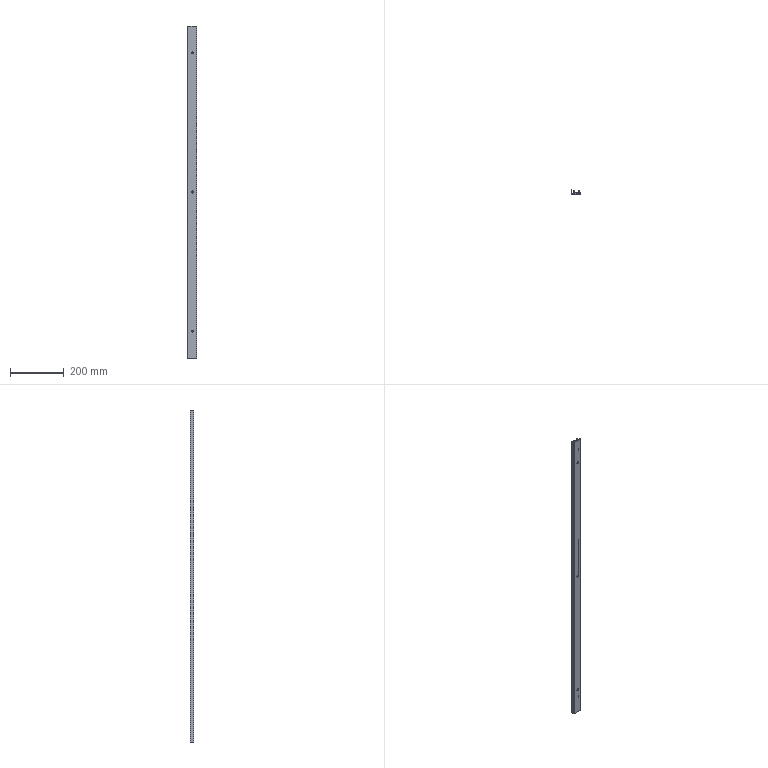Part | SolidWorks | features BaseBody 1, HoleWzd 1, ICE 1, MoveFace 1 | 1 solid | 31 faces | box 33.5 x 13.5 x 1230 mm | volume 229950 mm3 | plane 16 | cylinder 9 | cone 6 | commonest cylinder face diameters 2 x3 13.44 x3 4 x2 1.5 x1
STEP:
#1=CARTESIAN_POINT('',(20.,0.,1033.72));
#2=VERTEX_POINT('',#1);
#3=CARTESIAN_POINT('',(20.,0.,1026.28));
#4=VERTEX_POINT('',#3);
#5=CARTESIAN_POINT('',(20.,0.,1030.));
#6=DIRECTION('',(0.,-1.,0.));
#7=DIRECTION('',(0.,0.,-1.));
#8=AXIS2_PLACEMENT_3D('',#5,#6,#7);
#9=CIRCLE('',#8,3.72);
#10=EDGE_CURVE('',#2,#4,#9,.T.);
#11=ORIENTED_EDGE('',*,*,#10,.T.);
#12=CARTESIAN_POINT('',(20.,3.,1023.28));
#13=VERTEX_POINT('',#12);
#14=CARTESIAN_POINT('',(20.,3.,1023.28));
#15=DIRECTION('',(0.,0.7071,-0.7071));
#16=VECTOR('',#15,1000.);
#17=LINE('',#14,#16);
#18=EDGE_CURVE('',#4,#13,#17,.T.);
#19=ORIENTED_EDGE('',*,*,#18,.T.);
#20=CARTESIAN_POINT('',(20.,3.,1036.72));
#21=VERTEX_POINT('',#20);
#22=CARTESIAN_POINT('',(20.,3.,1030.));
#23=DIRECTION('',(0.,1.,0.));
#24=DIRECTION('',(0.,0.,1.));
#25=AXIS2_PLACEMENT_3D('',#22,#23,#24);
#26=CIRCLE('',#25,6.72);
#27=EDGE_CURVE('',#13,#21,#26,.T.);
#28=ORIENTED_EDGE('',*,*,#27,.T.);
#29=CARTESIAN_POINT('',(20.,3.,1036.72));
#30=DIRECTION('',(0.,0.7071,0.7071));
#31=VECTOR('',#30,1000.);
#32=LINE('',#29,#31);
#33=EDGE_CURVE('',#2,#21,#32,.T.);
#34=ORIENTED_EDGE('',*,*,#33,.F.);
#35=EDGE_LOOP('',(#11,#19,#28,#34));
#36=FACE_OUTER_BOUND('',#35,.T.);
#37=CARTESIAN_POINT('',(20.,3.,1030.));
#38=DIRECTION('',(0.,1.,0.));
#39=DIRECTION('',(0.,0.,1.));
#40=AXIS2_PLACEMENT_3D('',#37,#38,#39);
#41=CONICAL_SURFACE('',#40,6.72,0.7854);
#42=ADVANCED_FACE('',(#36),#41,.F.);
#43=CARTESIAN_POINT('',(20.,0.,3.72));
#44=VERTEX_POINT('',#43);
#45=CARTESIAN_POINT('',(20.,0.,-3.72));
#46=VERTEX_POINT('',#45);
#47=CARTESIAN_POINT('',(20.,0.,0.));
#48=DIRECTION('',(0.,-1.,0.));
#49=DIRECTION('',(0.,0.,-1.));
#50=AXIS2_PLACEMENT_3D('',#47,#48,#49);
#51=CIRCLE('',#50,3.72);
#52=EDGE_CURVE('',#44,#46,#51,.T.);
#53=ORIENTED_EDGE('',*,*,#52,.T.);
#54=CARTESIAN_POINT('',(20.,3.,-6.72));
#55=VERTEX_POINT('',#54);
#56=CARTESIAN_POINT('',(20.,3.,-6.72));
#57=DIRECTION('',(0.,0.7071,-0.7071));
#58=VECTOR('',#57,1000.);
#59=LINE('',#56,#58);
#60=EDGE_CURVE('',#46,#55,#59,.T.);
#61=ORIENTED_EDGE('',*,*,#60,.T.);
#62=CARTESIAN_POINT('',(20.,3.,6.72));
#63=VERTEX_POINT('',#62);
#64=CARTESIAN_POINT('',(20.,3.,0.));
#65=DIRECTION('',(0.,1.,0.));
#66=DIRECTION('',(0.,0.,1.));
#67=AXIS2_PLACEMENT_3D('',#64,#65,#66);
#68=CIRCLE('',#67,6.72);
#69=EDGE_CURVE('',#55,#63,#68,.T.);
#70=ORIENTED_EDGE('',*,*,#69,.T.);
#71=CARTESIAN_POINT('',(20.,3.,6.72));
#72=DIRECTION('',(0.,0.7071,0.7071));
#73=VECTOR('',#72,1000.);
#74=LINE('',#71,#73);
#75=EDGE_CURVE('',#44,#63,#74,.T.);
#76=ORIENTED_EDGE('',*,*,#75,.F.);
#77=EDGE_LOOP('',(#53,#61,#70,#76));
#78=FACE_OUTER_BOUND('',#77,.T.);
#79=CARTESIAN_POINT('',(20.,3.,0.));
#80=DIRECTION('',(0.,1.,0.));
#81=DIRECTION('',(0.,0.,1.));
#82=AXIS2_PLACEMENT_3D('',#79,#80,#81);
#83=CONICAL_SURFACE('',#82,6.72,0.7854);
#84=ADVANCED_FACE('',(#78),#83,.F.);
#85=CARTESIAN_POINT('',(20.,0.,518.72));
#86=VERTEX_POINT('',#85);
#87=CARTESIAN_POINT('',(20.,0.,511.28));
#88=VERTEX_POINT('',#87);
#89=CARTESIAN_POINT('',(20.,0.,515.));
#90=DIRECTION('',(0.,-1.,0.));
#91=DIRECTION('',(0.,0.,-1.));
#92=AXIS2_PLACEMENT_3D('',#89,#90,#91);
#93=CIRCLE('',#92,3.72);
#94=EDGE_CURVE('',#86,#88,#93,.T.);
#95=ORIENTED_EDGE('',*,*,#94,.T.);
#96=CARTESIAN_POINT('',(20.,3.,508.28));
#97=VERTEX_POINT('',#96);
#98=CARTESIAN_POINT('',(20.,3.,508.28));
#99=DIRECTION('',(0.,0.7071,-0.7071));
#100=VECTOR('',#99,1000.);
#101=LINE('',#98,#100);
#102=EDGE_CURVE('',#88,#97,#101,.T.);
#103=ORIENTED_EDGE('',*,*,#102,.T.);
#104=CARTESIAN_POINT('',(20.,3.,521.72));
#105=VERTEX_POINT('',#104);
#106=CARTESIAN_POINT('',(20.,3.,515.));
#107=DIRECTION('',(0.,1.,0.));
#108=DIRECTION('',(0.,0.,1.));
#109=AXIS2_PLACEMENT_3D('',#106,#107,#108);
#110=CIRCLE('',#109,6.72);
#111=EDGE_CURVE('',#97,#105,#110,.T.);
#112=ORIENTED_EDGE('',*,*,#111,.T.);
#113=CARTESIAN_POINT('',(20.,3.,521.72));
#114=DIRECTION('',(0.,0.7071,0.7071));
#115=VECTOR('',#114,1000.);
#116=LINE('',#113,#115);
#117=EDGE_CURVE('',#86,#105,#116,.T.);
#118=ORIENTED_EDGE('',*,*,#117,.F.);
#119=EDGE_LOOP('',(#95,#103,#112,#118));
#120=FACE_OUTER_BOUND('',#119,.T.);
#121=CARTESIAN_POINT('',(20.,3.,515.));
#122=DIRECTION('',(0.,1.,0.));
#123=DIRECTION('',(0.,0.,1.));
#124=AXIS2_PLACEMENT_3D('',#121,#122,#123);
#125=CONICAL_SURFACE('',#124,6.72,0.7854);
#126=ADVANCED_FACE('',(#120),#125,.F.);
#127=CARTESIAN_POINT('',(24.5,10.5,-4.991));
#128=VERTEX_POINT('',#127);
#129=CARTESIAN_POINT('',(24.5,10.5,-100.));
#130=VERTEX_POINT('',#129);
#131=CARTESIAN_POINT('',(24.5,10.5,-100.));
#132=DIRECTION('',(0.,0.,-1.));
#133=VECTOR('',#132,1000.);
#134=LINE('',#131,#133);
#135=EDGE_CURVE('',#128,#130,#134,.T.);
#136=ORIENTED_EDGE('',*,*,#135,.F.);
#137=CARTESIAN_POINT('',(24.5,10.5,4.991));
#138=VERTEX_POINT('',#137);
#139=CARTESIAN_POINT('',(24.5,10.5,-4.991));
#140=CARTESIAN_POINT('',(24.5,10.638,-4.991));
#141=CARTESIAN_POINT('',(24.515,10.777,-4.978));
#142=CARTESIAN_POINT('',(24.57,11.043,-4.927));
#143=CARTESIAN_POINT('',(24.611,11.171,-4.889));
#144=CARTESIAN_POINT('',(24.765,11.529,-4.74));
#145=CARTESIAN_POINT('',(24.907,11.728,-4.597));
#146=CARTESIAN_POINT('',(25.205,12.04,-4.256));
#147=CARTESIAN_POINT('',(25.365,12.156,-4.055));
#148=CARTESIAN_POINT('',(25.663,12.325,-3.627));
#149=CARTESIAN_POINT('',(25.806,12.38,-3.395));
#150=CARTESIAN_POINT('',(26.19,12.494,-2.672));
#151=CARTESIAN_POINT('',(26.387,12.501,-2.161));
#152=CARTESIAN_POINT('',(26.654,12.499,-1.091));
#153=CARTESIAN_POINT('',(26.72,12.488,-0.5481));
#154=CARTESIAN_POINT('',(26.72,12.488,0.2773));
#155=CARTESIAN_POINT('',(26.703,12.49,0.5529));
#156=CARTESIAN_POINT('',(26.636,12.496,1.095));
#157=CARTESIAN_POINT('',(26.586,12.499,1.362));
#158=CARTESIAN_POINT('',(26.388,12.501,2.155));
#159=CARTESIAN_POINT('',(26.188,12.493,2.677));
#160=CARTESIAN_POINT('',(25.805,12.38,3.396));
#161=CARTESIAN_POINT('',(25.662,12.324,3.629));
#162=CARTESIAN_POINT('',(25.438,12.197,3.95));
#163=CARTESIAN_POINT('',(25.362,12.147,4.053));
#164=CARTESIAN_POINT('',(25.208,12.03,4.249));
#165=CARTESIAN_POINT('',(25.13,11.961,4.342));
#166=CARTESIAN_POINT('',(24.98,11.805,4.513));
#167=CARTESIAN_POINT('',(24.908,11.717,4.591));
#168=CARTESIAN_POINT('',(24.774,11.518,4.73));
#169=CARTESIAN_POINT('',(24.714,11.408,4.79));
#170=CARTESIAN_POINT('',(24.612,11.172,4.888));
#171=CARTESIAN_POINT('',(24.57,11.043,4.927));
#172=CARTESIAN_POINT('',(24.515,10.778,4.978));
#173=CARTESIAN_POINT('',(24.5,10.64,4.991));
#174=CARTESIAN_POINT('',(24.5,10.5,4.991));
#175=B_SPLINE_CURVE_WITH_KNOTS('',3,(#139,#140,#141,#142,#143,#144,#145,#146,#147,#148,#149,#150,#151,#152,#153,#154,#155,#156,#157,#158,#159,#160,#161,#162,#163,#164,#165,#166,#167,#168,#169,#170,#171,#172,#173,#174),.UNSPECIFIED.,.F.,.F.,(4,2,2,2,2,2,2,2,2,2,2,2,2,2,2,2,2,4),(0.01321,0.01362,0.01403,0.01486,0.01569,0.01651,0.01816,0.01981,0.02064,0.02146,0.02311,0.02394,0.02435,0.02477,0.02518,0.02559,0.026,0.02642),.UNSPECIFIED.);
#176=EDGE_CURVE('',#128,#138,#175,.T.);
#177=ORIENTED_EDGE('',*,*,#176,.T.);
#178=CARTESIAN_POINT('',(24.5,10.5,510.009));
#179=VERTEX_POINT('',#178);
#180=CARTESIAN_POINT('',(24.5,10.5,-100.));
#181=DIRECTION('',(0.,0.,-1.));
#182=VECTOR('',#181,1000.);
#183=LINE('',#180,#182);
#184=EDGE_CURVE('',#179,#138,#183,.T.);
#185=ORIENTED_EDGE('',*,*,#184,.F.);
#186=CARTESIAN_POINT('',(24.5,10.5,519.991));
#187=VERTEX_POINT('',#186);
#188=CARTESIAN_POINT('',(24.5,10.5,510.009));
#189=CARTESIAN_POINT('',(24.5,10.638,510.009));
#190=CARTESIAN_POINT('',(24.515,10.777,510.022));
#191=CARTESIAN_POINT('',(24.57,11.043,510.073));
#192=CARTESIAN_POINT('',(24.611,11.171,510.111));
#193=CARTESIAN_POINT('',(24.765,11.529,510.26));
#194=CARTESIAN_POINT('',(24.907,11.728,510.403));
#195=CARTESIAN_POINT('',(25.205,12.04,510.744));
#196=CARTESIAN_POINT('',(25.365,12.156,510.945));
#197=CARTESIAN_POINT('',(25.663,12.325,511.373));
#198=CARTESIAN_POINT('',(25.806,12.38,511.605));
#199=CARTESIAN_POINT('',(26.19,12.494,512.328));
#200=CARTESIAN_POINT('',(26.387,12.501,512.839));
#201=CARTESIAN_POINT('',(26.654,12.499,513.909));
#202=CARTESIAN_POINT('',(26.72,12.488,514.452));
#203=CARTESIAN_POINT('',(26.72,12.488,515.277));
#204=CARTESIAN_POINT('',(26.703,12.49,515.553));
#205=CARTESIAN_POINT('',(26.636,12.496,516.095));
#206=CARTESIAN_POINT('',(26.586,12.499,516.362));
#207=CARTESIAN_POINT('',(26.388,12.501,517.155));
#208=CARTESIAN_POINT('',(26.188,12.493,517.677));
#209=CARTESIAN_POINT('',(25.805,12.38,518.396));
#210=CARTESIAN_POINT('',(25.662,12.324,518.629));
#211=CARTESIAN_POINT('',(25.438,12.197,518.95));
#212=CARTESIAN_POINT('',(25.362,12.147,519.053));
#213=CARTESIAN_POINT('',(25.208,12.03,519.249));
#214=CARTESIAN_POINT('',(25.13,11.961,519.342));
#215=CARTESIAN_POINT('',(24.98,11.805,519.513));
#216=CARTESIAN_POINT('',(24.908,11.717,519.591));
#217=CARTESIAN_POINT('',(24.774,11.518,519.73));
#218=CARTESIAN_POINT('',(24.714,11.408,519.79));
#219=CARTESIAN_POINT('',(24.612,11.172,519.888));
#220=CARTESIAN_POINT('',(24.57,11.043,519.927));
#221=CARTESIAN_POINT('',(24.515,10.778,519.978));
#222=CARTESIAN_POINT('',(24.5,10.64,519.991));
#223=CARTESIAN_POINT('',(24.5,10.5,519.991));
#224=B_SPLINE_CURVE_WITH_KNOTS('',3,(#188,#189,#190,#191,#192,#193,#194,#195,#196,#197,#198,#199,#200,#201,#202,#203,#204,#205,#206,#207,#208,#209,#210,#211,#212,#213,#214,#215,#216,#217,#218,#219,#220,#221,#222,#223),.UNSPECIFIED.,.F.,.F.,(4,2,2,2,2,2,2,2,2,2,2,2,2,2,2,2,2,4),(0.01321,0.01362,0.01403,0.01486,0.01569,0.01651,0.01816,0.01981,0.02064,0.02146,0.02311,0.02394,0.02435,0.02477,0.02518,0.02559,0.026,0.02642),.UNSPECIFIED.);
#225=EDGE_CURVE('',#179,#187,#224,.T.);
#226=ORIENTED_EDGE('',*,*,#225,.T.);
#227=CARTESIAN_POINT('',(24.5,10.5,1025.009));
#228=VERTEX_POINT('',#227);
#229=CARTESIAN_POINT('',(24.5,10.5,-100.));
#230=DIRECTION('',(0.,0.,-1.));
#231=VECTOR('',#230,1000.);
#232=LINE('',#229,#231);
#233=EDGE_CURVE('',#228,#187,#232,.T.);
#234=ORIENTED_EDGE('',*,*,#233,.F.);
#235=CARTESIAN_POINT('',(24.5,10.5,1034.991));
#236=VERTEX_POINT('',#235);
#237=CARTESIAN_POINT('',(24.5,10.5,1025.009));
#238=CARTESIAN_POINT('',(24.5,10.64,1025.009));
#239=CARTESIAN_POINT('',(24.514,10.776,1025.022));
#240=CARTESIAN_POINT('',(24.57,11.042,1025.073));
#241=CARTESIAN_POINT('',(24.611,11.171,1025.111));
#242=CARTESIAN_POINT('',(24.713,11.408,1025.209));
#243=CARTESIAN_POINT('',(24.775,11.519,1025.27));
#244=CARTESIAN_POINT('',(24.908,11.717,1025.409));
#245=CARTESIAN_POINT('',(24.981,11.806,1025.488));
#246=CARTESIAN_POINT('',(25.207,12.042,1025.746));
#247=CARTESIAN_POINT('',(25.363,12.155,1025.942));
#248=CARTESIAN_POINT('',(25.665,12.326,1026.376));
#249=CARTESIAN_POINT('',(25.806,12.38,1026.605));
#250=CARTESIAN_POINT('',(26.061,12.456,1027.084));
#251=CARTESIAN_POINT('',(26.176,12.476,1027.337));
#252=CARTESIAN_POINT('',(26.372,12.498,1027.849));
#253=CARTESIAN_POINT('',(26.454,12.501,1028.109));
#254=CARTESIAN_POINT('',(26.586,12.499,1028.638));
#255=CARTESIAN_POINT('',(26.636,12.496,1028.907));
#256=CARTESIAN_POINT('',(26.703,12.49,1029.453));
#257=CARTESIAN_POINT('',(26.72,12.488,1029.729));
#258=CARTESIAN_POINT('',(26.72,12.488,1030.275));
#259=CARTESIAN_POINT('',(26.703,12.49,1030.547));
#260=CARTESIAN_POINT('',(26.637,12.496,1031.089));
#261=CARTESIAN_POINT('',(26.587,12.499,1031.36));
#262=CARTESIAN_POINT('',(26.387,12.501,1032.161));
#263=CARTESIAN_POINT('',(26.191,12.494,1032.671));
#264=CARTESIAN_POINT('',(25.805,12.38,1033.396));
#265=CARTESIAN_POINT('',(25.663,12.325,1033.627));
#266=CARTESIAN_POINT('',(25.364,12.155,1034.057));
#267=CARTESIAN_POINT('',(25.205,12.039,1034.256));
#268=CARTESIAN_POINT('',(24.981,11.805,1034.512));
#269=CARTESIAN_POINT('',(24.907,11.716,1034.592));
#270=CARTESIAN_POINT('',(24.774,11.518,1034.73));
#271=CARTESIAN_POINT('',(24.714,11.409,1034.79));
#272=CARTESIAN_POINT('',(24.611,11.17,1034.889));
#273=CARTESIAN_POINT('',(24.571,11.044,1034.926));
#274=CARTESIAN_POINT('',(24.515,10.78,1034.977));
#275=CARTESIAN_POINT('',(24.5,10.64,1034.991));
#276=CARTESIAN_POINT('',(24.5,10.5,1034.991));
#277=B_SPLINE_CURVE_WITH_KNOTS('',3,(#237,#238,#239,#240,#241,#242,#243,#244,#245,#246,#247,#248,#249,#250,#251,#252,#253,#254,#255,#256,#257,#258,#259,#260,#261,#262,#263,#264,#265,#266,#267,#268,#269,#270,#271,#272,#273,#274,#275,#276),.UNSPECIFIED.,.F.,.F.,(4,2,2,2,2,2,2,2,2,2,2,2,2,2,2,2,2,2,2,4),(0.,0.0004127,0.0008255,0.001238,0.001651,0.002476,0.003302,0.004127,0.004953,0.005778,0.006604,0.007429,0.008255,0.009906,0.01073,0.01156,0.01197,0.01238,0.01279,0.01321),.UNSPECIFIED.);
#278=EDGE_CURVE('',#228,#236,#277,.T.);
#279=ORIENTED_EDGE('',*,*,#278,.T.);
#280=CARTESIAN_POINT('',(24.5,10.5,1130.));
#281=VERTEX_POINT('',#280);
#282=CARTESIAN_POINT('',(24.5,10.5,-100.));
#283=DIRECTION('',(0.,0.,-1.));
#284=VECTOR('',#283,1000.);
#285=LINE('',#282,#284);
#286=EDGE_CURVE('',#281,#236,#285,.T.);
#287=ORIENTED_EDGE('',*,*,#286,.F.);
#288=CARTESIAN_POINT('',(28.5,10.5,1130.));
#289=VERTEX_POINT('',#288);
#290=CARTESIAN_POINT('',(26.5,10.5,1130.));
#291=DIRECTION('',(0.,0.,1.));
#292=DIRECTION('',(1.,0.,0.));
#293=AXIS2_PLACEMENT_3D('',#290,#291,#292);
#294=CIRCLE('',#293,2.);
#295=EDGE_CURVE('',#289,#281,#294,.T.);
#296=ORIENTED_EDGE('',*,*,#295,.F.);
#297=CARTESIAN_POINT('',(28.5,10.5,-100.));
#298=VERTEX_POINT('',#297);
#299=CARTESIAN_POINT('',(28.5,10.5,-100.));
#300=DIRECTION('',(0.,0.,-1.));
#301=VECTOR('',#300,1000.);
#302=LINE('',#299,#301);
#303=EDGE_CURVE('',#289,#298,#302,.T.);
#304=ORIENTED_EDGE('',*,*,#303,.T.);
#305=CARTESIAN_POINT('',(26.5,10.5,-100.));
#306=DIRECTION('',(0.,0.,1.));
#307=DIRECTION('',(-1.,0.,0.));
#308=AXIS2_PLACEMENT_3D('',#305,#306,#307);
#309=CIRCLE('',#308,2.);
#310=EDGE_CURVE('',#298,#130,#309,.T.);
#311=ORIENTED_EDGE('',*,*,#310,.T.);
#312=EDGE_LOOP('',(#136,#177,#185,#226,#234,#279,#287,#296,#304,#311));
#313=FACE_OUTER_BOUND('',#312,.T.);
#314=CARTESIAN_POINT('',(26.5,10.5,-100.));
#315=DIRECTION('',(0.,0.,-1.));
#316=DIRECTION('',(-1.,0.,0.));
#317=AXIS2_PLACEMENT_3D('',#314,#315,#316);
#318=CYLINDRICAL_SURFACE('',#317,2.);
#319=ADVANCED_FACE('',(#313),#318,.T.);
#320=CARTESIAN_POINT('',(24.5,3.,-4.991));
#321=VERTEX_POINT('',#320);
#322=CARTESIAN_POINT('',(24.5,3.,-100.));
#323=VERTEX_POINT('',#322);
#324=CARTESIAN_POINT('',(24.5,3.,-100.));
#325=DIRECTION('',(0.,0.,-1.));
#326=VECTOR('',#325,1000.);
#327=LINE('',#324,#326);
#328=EDGE_CURVE('',#321,#323,#327,.T.);
#329=ORIENTED_EDGE('',*,*,#328,.F.);
#330=CARTESIAN_POINT('',(24.5,13.5,-4.991));
#331=DIRECTION('',(0.,1.,0.));
#332=VECTOR('',#331,1000.);
#333=LINE('',#330,#332);
#334=EDGE_CURVE('',#321,#128,#333,.T.);
#335=ORIENTED_EDGE('',*,*,#334,.T.);
#336=ORIENTED_EDGE('',*,*,#135,.T.);
#337=CARTESIAN_POINT('',(24.5,1.,-100.));
#338=DIRECTION('',(0.,-1.,0.));
#339=VECTOR('',#338,1000.);
#340=LINE('',#337,#339);
#341=EDGE_CURVE('',#130,#323,#340,.T.);
#342=ORIENTED_EDGE('',*,*,#341,.T.);
#343=EDGE_LOOP('',(#329,#335,#336,#342));
#344=FACE_OUTER_BOUND('',#343,.T.);
#345=CARTESIAN_POINT('',(24.5,10.5,-100.));
#346=DIRECTION('',(-1.,0.,0.));
#347=DIRECTION('',(0.,0.,1.));
#348=AXIS2_PLACEMENT_3D('',#345,#346,#347);
#349=PLANE('',#348);
#350=ADVANCED_FACE('',(#344),#349,.T.);
#351=ORIENTED_EDGE('',*,*,#184,.T.);
#352=CARTESIAN_POINT('',(24.5,3.,4.991));
#353=VERTEX_POINT('',#352);
#354=CARTESIAN_POINT('',(24.5,13.5,4.991));
#355=DIRECTION('',(0.,-1.,0.));
#356=VECTOR('',#355,1000.);
#357=LINE('',#354,#356);
#358=EDGE_CURVE('',#138,#353,#357,.T.);
#359=ORIENTED_EDGE('',*,*,#358,.T.);
#360=CARTESIAN_POINT('',(24.5,3.,510.009));
#361=VERTEX_POINT('',#360);
#362=CARTESIAN_POINT('',(24.5,3.,-100.));
#363=DIRECTION('',(0.,0.,-1.));
#364=VECTOR('',#363,1000.);
#365=LINE('',#362,#364);
#366=EDGE_CURVE('',#361,#353,#365,.T.);
#367=ORIENTED_EDGE('',*,*,#366,.F.);
#368=CARTESIAN_POINT('',(24.5,13.5,510.009));
#369=DIRECTION('',(0.,1.,0.));
#370=VECTOR('',#369,1000.);
#371=LINE('',#368,#370);
#372=EDGE_CURVE('',#361,#179,#371,.T.);
#373=ORIENTED_EDGE('',*,*,#372,.T.);
#374=EDGE_LOOP('',(#351,#359,#367,#373));
#375=FACE_OUTER_BOUND('',#374,.T.);
#376=CARTESIAN_POINT('',(24.5,10.5,-100.));
#377=DIRECTION('',(-1.,0.,0.));
#378=DIRECTION('',(0.,0.,1.));
#379=AXIS2_PLACEMENT_3D('',#376,#377,#378);
#380=PLANE('',#379);
#381=ADVANCED_FACE('',(#375),#380,.T.);
#382=ORIENTED_EDGE('',*,*,#233,.T.);
#383=CARTESIAN_POINT('',(24.5,3.,519.991));
#384=VERTEX_POINT('',#383);
#385=CARTESIAN_POINT('',(24.5,13.5,519.991));
#386=DIRECTION('',(0.,-1.,0.));
#387=VECTOR('',#386,1000.);
#388=LINE('',#385,#387);
#389=EDGE_CURVE('',#187,#384,#388,.T.);
#390=ORIENTED_EDGE('',*,*,#389,.T.);
#391=CARTESIAN_POINT('',(24.5,3.,1025.009));
#392=VERTEX_POINT('',#391);
#393=CARTESIAN_POINT('',(24.5,3.,-100.));
#394=DIRECTION('',(0.,0.,-1.));
#395=VECTOR('',#394,1000.);
#396=LINE('',#393,#395);
#397=EDGE_CURVE('',#392,#384,#396,.T.);
#398=ORIENTED_EDGE('',*,*,#397,.F.);
#399=CARTESIAN_POINT('',(24.5,13.5,1025.009));
#400=DIRECTION('',(0.,1.,0.));
#401=VECTOR('',#400,1000.);
#402=LINE('',#399,#401);
#403=EDGE_CURVE('',#392,#228,#402,.T.);
#404=ORIENTED_EDGE('',*,*,#403,.T.);
#405=EDGE_LOOP('',(#382,#390,#398,#404));
#406=FACE_OUTER_BOUND('',#405,.T.);
#407=CARTESIAN_POINT('',(24.5,10.5,-100.));
#408=DIRECTION('',(-1.,0.,0.));
#409=DIRECTION('',(0.,0.,1.));
#410=AXIS2_PLACEMENT_3D('',#407,#408,#409);
#411=PLANE('',#410);
#412=ADVANCED_FACE('',(#406),#411,.T.);
#413=ORIENTED_EDGE('',*,*,#286,.T.);
#414=CARTESIAN_POINT('',(24.5,3.,1034.991));
#415=VERTEX_POINT('',#414);
#416=CARTESIAN_POINT('',(24.5,13.5,1034.991));
#417=DIRECTION('',(0.,-1.,0.));
#418=VECTOR('',#417,1000.);
#419=LINE('',#416,#418);
#420=EDGE_CURVE('',#236,#415,#419,.T.);
#421=ORIENTED_EDGE('',*,*,#420,.T.);
#422=CARTESIAN_POINT('',(24.5,3.,1130.));
#423=VERTEX_POINT('',#422);
#424=CARTESIAN_POINT('',(24.5,3.,-100.));
#425=DIRECTION('',(0.,0.,-1.));
#426=VECTOR('',#425,1000.);
#427=LINE('',#424,#426);
#428=EDGE_CURVE('',#423,#415,#427,.T.);
#429=ORIENTED_EDGE('',*,*,#428,.F.);
#430=CARTESIAN_POINT('',(24.5,1.,1130.));
#431=DIRECTION('',(0.,-1.,0.));
#432=VECTOR('',#431,1000.);
#433=LINE('',#430,#432);
#434=EDGE_CURVE('',#281,#423,#433,.T.);
#435=ORIENTED_EDGE('',*,*,#434,.F.);
#436=EDGE_LOOP('',(#413,#421,#429,#435));
#437=FACE_OUTER_BOUND('',#436,.T.);
#438=CARTESIAN_POINT('',(24.5,10.5,-100.));
#439=DIRECTION('',(-1.,0.,0.));
#440=DIRECTION('',(0.,0.,1.));
#441=AXIS2_PLACEMENT_3D('',#438,#439,#440);
#442=PLANE('',#441);
#443=ADVANCED_FACE('',(#437),#442,.T.);
#444=ORIENTED_EDGE('',*,*,#10,.F.);
#445=CARTESIAN_POINT('',(20.,0.,1030.));
#446=DIRECTION('',(0.,-1.,0.));
#447=DIRECTION('',(0.,0.,-1.));
#448=AXIS2_PLACEMENT_3D('',#445,#446,#447);
#449=CIRCLE('',#448,3.72);
#450=EDGE_CURVE('',#4,#2,#449,.T.);
#451=ORIENTED_EDGE('',*,*,#450,.F.);
#452=EDGE_LOOP('',(#444,#451));
#453=FACE_BOUND('',#452,.T.);
#454=ORIENTED_EDGE('',*,*,#94,.F.);
#455=CARTESIAN_POINT('',(20.,0.,515.));
#456=DIRECTION('',(0.,-1.,0.));
#457=DIRECTION('',(0.,0.,-1.));
#458=AXIS2_PLACEMENT_3D('',#455,#456,#457);
#459=CIRCLE('',#458,3.72);
#460=EDGE_CURVE('',#88,#86,#459,.T.);
#461=ORIENTED_EDGE('',*,*,#460,.F.);
#462=EDGE_LOOP('',(#454,#461));
#463=FACE_BOUND('',#462,.T.);
#464=CARTESIAN_POINT('',(1.,0.,-100.));
#465=VERTEX_POINT('',#464);
#466=CARTESIAN_POINT('',(32.5,0.,-100.));
#467=VERTEX_POINT('',#466);
#468=CARTESIAN_POINT('',(1.,0.,-100.));
#469=DIRECTION('',(1.,0.,0.));
#470=VECTOR('',#469,1000.);
#471=LINE('',#468,#470);
#472=EDGE_CURVE('',#465,#467,#471,.T.);
#473=ORIENTED_EDGE('',*,*,#472,.T.);
#474=CARTESIAN_POINT('',(32.5,0.,1130.));
#475=VERTEX_POINT('',#474);
#476=CARTESIAN_POINT('',(32.5,0.,-100.));
#477=DIRECTION('',(0.,0.,1.));
#478=VECTOR('',#477,1000.);
#479=LINE('',#476,#478);
#480=EDGE_CURVE('',#467,#475,#479,.T.);
#481=ORIENTED_EDGE('',*,*,#480,.T.);
#482=CARTESIAN_POINT('',(1.,0.,1130.));
#483=VERTEX_POINT('',#482);
#484=CARTESIAN_POINT('',(1.,0.,1130.));
#485=DIRECTION('',(-1.,0.,0.));
#486=VECTOR('',#485,1000.);
#487=LINE('',#484,#486);
#488=EDGE_CURVE('',#475,#483,#487,.T.);
#489=ORIENTED_EDGE('',*,*,#488,.T.);
#490=CARTESIAN_POINT('',(1.,0.,-100.));
#491=DIRECTION('',(0.,0.,-1.));
#492=VECTOR('',#491,1000.);
#493=LINE('',#490,#492);
#494=EDGE_CURVE('',#483,#465,#493,.T.);
#495=ORIENTED_EDGE('',*,*,#494,.T.);
#496=EDGE_LOOP('',(#473,#481,#489,#495));
#497=FACE_OUTER_BOUND('',#496,.T.);
#498=ORIENTED_EDGE('',*,*,#52,.F.);
#499=CARTESIAN_POINT('',(20.,0.,0.));
#500=DIRECTION('',(0.,-1.,0.));
#501=DIRECTION('',(0.,0.,-1.));
#502=AXIS2_PLACEMENT_3D('',#499,#500,#501);
#503=CIRCLE('',#502,3.72);
#504=EDGE_CURVE('',#46,#44,#503,.T.);
#505=ORIENTED_EDGE('',*,*,#504,.F.);
#506=EDGE_LOOP('',(#498,#505));
#507=FACE_BOUND('',#506,.T.);
#508=CARTESIAN_POINT('',(1.,0.,-100.));
#509=DIRECTION('',(0.,-1.,0.));
#510=DIRECTION('',(0.,0.,-1.));
#511=AXIS2_PLACEMENT_3D('',#508,#509,#510);
#512=PLANE('',#511);
#513=ADVANCED_FACE('',(#453,#463,#497,#507),#512,.T.);
#514=CARTESIAN_POINT('',(33.5,1.,-100.));
#515=VERTEX_POINT('',#514);
#516=CARTESIAN_POINT('',(32.5,1.,-100.));
#517=DIRECTION('',(0.,0.,1.));
#518=DIRECTION('',(-1.,0.,0.));
#519=AXIS2_PLACEMENT_3D('',#516,#517,#518);
#520=CIRCLE('',#519,1.);
#521=EDGE_CURVE('',#467,#515,#520,.T.);
#522=ORIENTED_EDGE('',*,*,#521,.T.);
#523=CARTESIAN_POINT('',(33.5,1.,1130.));
#524=VERTEX_POINT('',#523);
#525=CARTESIAN_POINT('',(33.5,1.,-100.));
#526=DIRECTION('',(0.,0.,1.));
#527=VECTOR('',#526,1000.);
#528=LINE('',#525,#527);
#529=EDGE_CURVE('',#515,#524,#528,.T.);
#530=ORIENTED_EDGE('',*,*,#529,.T.);
#531=CARTESIAN_POINT('',(32.5,1.,1130.));
#532=DIRECTION('',(0.,0.,-1.));
#533=DIRECTION('',(1.,0.,0.));
#534=AXIS2_PLACEMENT_3D('',#531,#532,#533);
#535=CIRCLE('',#534,1.);
#536=EDGE_CURVE('',#524,#475,#535,.T.);
#537=ORIENTED_EDGE('',*,*,#536,.T.);
#538=ORIENTED_EDGE('',*,*,#480,.F.);
#539=EDGE_LOOP('',(#522,#530,#537,#538));
#540=FACE_OUTER_BOUND('',#539,.T.);
#541=CARTESIAN_POINT('',(32.5,1.,-100.));
#542=DIRECTION('',(0.,0.,-1.));
#543=DIRECTION('',(-1.,0.,0.));
#544=AXIS2_PLACEMENT_3D('',#541,#542,#543);
#545=CYLINDRICAL_SURFACE('',#544,1.);
#546=ADVANCED_FACE('',(#540),#545,.T.);
#547=CARTESIAN_POINT('',(1.5,12.75,-100.));
#548=VERTEX_POINT('',#547);
#549=CARTESIAN_POINT('',(0.,12.75,-100.));
#550=VERTEX_POINT('',#549);
#551=CARTESIAN_POINT('',(0.75,12.75,-100.));
#552=DIRECTION('',(0.,0.,1.));
#553=DIRECTION('',(-1.,0.,0.));
#554=AXIS2_PLACEMENT_3D('',#551,#552,#553);
#555=CIRCLE('',#554,0.75);
#556=EDGE_CURVE('',#548,#550,#555,.T.);
#557=ORIENTED_EDGE('',*,*,#556,.F.);
#558=CARTESIAN_POINT('',(1.5,3.,-100.));
#559=VERTEX_POINT('',#558);
#560=CARTESIAN_POINT('',(1.5,1.,-100.));
#561=DIRECTION('',(0.,1.,0.));
#562=VECTOR('',#561,1000.);
#563=LINE('',#560,#562);
#564=EDGE_CURVE('',#559,#548,#563,.T.);
#565=ORIENTED_EDGE('',*,*,#564,.F.);
#566=CARTESIAN_POINT('',(8.5,3.,-100.));
#567=VERTEX_POINT('',#566);
#568=CARTESIAN_POINT('',(1.,3.,-100.));
#569=DIRECTION('',(-1.,0.,0.));
#570=VECTOR('',#569,1000.);
#571=LINE('',#568,#570);
#572=EDGE_CURVE('',#567,#559,#571,.T.);
#573=ORIENTED_EDGE('',*,*,#572,.F.);
#574=CARTESIAN_POINT('',(8.5,10.5,-100.));
#575=VERTEX_POINT('',#574);
#576=CARTESIAN_POINT('',(8.5,1.,-100.));
#577=DIRECTION('',(0.,-1.,0.));
#578=VECTOR('',#577,1000.);
#579=LINE('',#576,#578);
#580=EDGE_CURVE('',#575,#567,#579,.T.);
#581=ORIENTED_EDGE('',*,*,#580,.F.);
#582=CARTESIAN_POINT('',(12.5,10.5,-100.));
#583=VERTEX_POINT('',#582);
#584=CARTESIAN_POINT('',(10.5,10.5,-100.));
#585=DIRECTION('',(0.,0.,1.));
#586=DIRECTION('',(-1.,0.,0.));
#587=AXIS2_PLACEMENT_3D('',#584,#585,#586);
#588=CIRCLE('',#587,2.);
#589=EDGE_CURVE('',#583,#575,#588,.T.);
#590=ORIENTED_EDGE('',*,*,#589,.F.);
#591=CARTESIAN_POINT('',(12.5,3.,-100.));
#592=VERTEX_POINT('',#591);
#593=CARTESIAN_POINT('',(12.5,1.,-100.));
#594=DIRECTION('',(0.,1.,0.));
#595=VECTOR('',#594,1000.);
#596=LINE('',#593,#595);
#597=EDGE_CURVE('',#592,#583,#596,.T.);
#598=ORIENTED_EDGE('',*,*,#597,.F.);
#599=CARTESIAN_POINT('',(1.,3.,-100.));
#600=DIRECTION('',(-1.,0.,0.));
#601=VECTOR('',#600,1000.);
#602=LINE('',#599,#601);
#603=EDGE_CURVE('',#323,#592,#602,.T.);
#604=ORIENTED_EDGE('',*,*,#603,.F.);
#605=ORIENTED_EDGE('',*,*,#341,.F.);
#606=ORIENTED_EDGE('',*,*,#310,.F.);
#607=CARTESIAN_POINT('',(28.5,3.,-100.));
#608=VERTEX_POINT('',#607);
#609=CARTESIAN_POINT('',(28.5,1.,-100.));
#610=DIRECTION('',(0.,1.,0.));
#611=VECTOR('',#610,1000.);
#612=LINE('',#609,#611);
#613=EDGE_CURVE('',#608,#298,#612,.T.);
#614=ORIENTED_EDGE('',*,*,#613,.F.);
#615=CARTESIAN_POINT('',(32.5,3.,-100.));
#616=VERTEX_POINT('',#615);
#617=CARTESIAN_POINT('',(1.,3.,-100.));
#618=DIRECTION('',(-1.,0.,0.));
#619=VECTOR('',#618,1000.);
#620=LINE('',#617,#619);
#621=EDGE_CURVE('',#616,#608,#620,.T.);
#622=ORIENTED_EDGE('',*,*,#621,.F.);
#623=CARTESIAN_POINT('',(33.5,2.,-100.));
#624=VERTEX_POINT('',#623);
#625=CARTESIAN_POINT('',(32.5,2.,-100.));
#626=DIRECTION('',(0.,0.,1.));
#627=DIRECTION('',(-1.,0.,0.));
#628=AXIS2_PLACEMENT_3D('',#625,#626,#627);
#629=CIRCLE('',#628,1.);
#630=EDGE_CURVE('',#624,#616,#629,.T.);
#631=ORIENTED_EDGE('',*,*,#630,.F.);
#632=CARTESIAN_POINT('',(33.5,1.,-100.));
#633=DIRECTION('',(0.,1.,0.));
#634=VECTOR('',#633,1000.);
#635=LINE('',#632,#634);
#636=EDGE_CURVE('',#515,#624,#635,.T.);
#637=ORIENTED_EDGE('',*,*,#636,.F.);
#638=ORIENTED_EDGE('',*,*,#521,.F.);
#639=ORIENTED_EDGE('',*,*,#472,.F.);
#640=CARTESIAN_POINT('',(0.,1.,-100.));
#641=VERTEX_POINT('',#640);
#642=CARTESIAN_POINT('',(1.,1.,-100.));
#643=DIRECTION('',(0.,0.,1.));
#644=DIRECTION('',(-1.,0.,0.));
#645=AXIS2_PLACEMENT_3D('',#642,#643,#644);
#646=CIRCLE('',#645,1.);
#647=EDGE_CURVE('',#641,#465,#646,.T.);
#648=ORIENTED_EDGE('',*,*,#647,.F.);
#649=CARTESIAN_POINT('',(0.,1.,-100.));
#650=DIRECTION('',(0.,-1.,0.));
#651=VECTOR('',#650,1000.);
#652=LINE('',#649,#651);
#653=EDGE_CURVE('',#550,#641,#652,.T.);
#654=ORIENTED_EDGE('',*,*,#653,.F.);
#655=EDGE_LOOP('',(#557,#565,#573,#581,#590,#598,#604,#605,#606,#614,#622,#631,#637,#638,#639,#648,#654));
#656=FACE_OUTER_BOUND('',#655,.T.);
#657=CARTESIAN_POINT('',(1.,1.,-100.));
#658=DIRECTION('',(0.,0.,1.));
#659=DIRECTION('',(1.,0.,0.));
#660=AXIS2_PLACEMENT_3D('',#657,#658,#659);
#661=PLANE('',#660);
#662=ADVANCED_FACE('',(#656),#661,.F.);
#663=ORIENTED_EDGE('',*,*,#647,.T.);
#664=ORIENTED_EDGE('',*,*,#494,.F.);
#665=CARTESIAN_POINT('',(0.,1.,1130.));
#666=VERTEX_POINT('',#665);
#667=CARTESIAN_POINT('',(1.,1.,1130.));
#668=DIRECTION('',(0.,0.,-1.));
#669=DIRECTION('',(1.,0.,0.));
#670=AXIS2_PLACEMENT_3D('',#667,#668,#669);
#671=CIRCLE('',#670,1.);
#672=EDGE_CURVE('',#483,#666,#671,.T.);
#673=ORIENTED_EDGE('',*,*,#672,.T.);
#674=CARTESIAN_POINT('',(0.,1.,-100.));
#675=DIRECTION('',(0.,0.,-1.));
#676=VECTOR('',#675,1000.);
#677=LINE('',#674,#676);
#678=EDGE_CURVE('',#666,#641,#677,.T.);
#679=ORIENTED_EDGE('',*,*,#678,.T.);
#680=EDGE_LOOP('',(#663,#664,#673,#679));
#681=FACE_OUTER_BOUND('',#680,.T.);
#682=CARTESIAN_POINT('',(1.,1.,-100.));
#683=DIRECTION('',(0.,0.,-1.));
#684=DIRECTION('',(-1.,0.,0.));
#685=AXIS2_PLACEMENT_3D('',#682,#683,#684);
#686=CYLINDRICAL_SURFACE('',#685,1.);
#687=ADVANCED_FACE('',(#681),#686,.T.);
#688=CARTESIAN_POINT('',(1.5,3.,1130.));
#689=VERTEX_POINT('',#688);
#690=CARTESIAN_POINT('',(1.5,12.75,1130.));
#691=VERTEX_POINT('',#690);
#692=CARTESIAN_POINT('',(1.5,1.,1130.));
#693=DIRECTION('',(0.,1.,0.));
#694=VECTOR('',#693,1000.);
#695=LINE('',#692,#694);
#696=EDGE_CURVE('',#689,#691,#695,.T.);
#697=ORIENTED_EDGE('',*,*,#696,.T.);
#698=CARTESIAN_POINT('',(0.,12.75,1130.));
#699=VERTEX_POINT('',#698);
#700=CARTESIAN_POINT('',(0.75,12.75,1130.));
#701=DIRECTION('',(0.,0.,1.));
#702=DIRECTION('',(1.,0.,0.));
#703=AXIS2_PLACEMENT_3D('',#700,#701,#702);
#704=CIRCLE('',#703,0.75);
#705=EDGE_CURVE('',#691,#699,#704,.T.);
#706=ORIENTED_EDGE('',*,*,#705,.T.);
#707=CARTESIAN_POINT('',(0.,1.,1130.));
#708=DIRECTION('',(0.,-1.,0.));
#709=VECTOR('',#708,1000.);
#710=LINE('',#707,#709);
#711=EDGE_CURVE('',#699,#666,#710,.T.);
#712=ORIENTED_EDGE('',*,*,#711,.T.);
#713=ORIENTED_EDGE('',*,*,#672,.F.);
#714=ORIENTED_EDGE('',*,*,#488,.F.);
#715=ORIENTED_EDGE('',*,*,#536,.F.);
#716=CARTESIAN_POINT('',(33.5,2.,1130.));
#717=VERTEX_POINT('',#716);
#718=CARTESIAN_POINT('',(33.5,1.,1130.));
#719=DIRECTION('',(0.,1.,0.));
#720=VECTOR('',#719,1000.);
#721=LINE('',#718,#720);
#722=EDGE_CURVE('',#524,#717,#721,.T.);
#723=ORIENTED_EDGE('',*,*,#722,.T.);
#724=CARTESIAN_POINT('',(32.5,3.,1130.));
#725=VERTEX_POINT('',#724);
#726=CARTESIAN_POINT('',(32.5,2.,1130.));
#727=DIRECTION('',(0.,0.,-1.));
#728=DIRECTION('',(1.,0.,0.));
#729=AXIS2_PLACEMENT_3D('',#726,#727,#728);
#730=CIRCLE('',#729,1.);
#731=EDGE_CURVE('',#725,#717,#730,.T.);
#732=ORIENTED_EDGE('',*,*,#731,.F.);
#733=CARTESIAN_POINT('',(28.5,3.,1130.));
#734=VERTEX_POINT('',#733);
#735=CARTESIAN_POINT('',(1.,3.,1130.));
#736=DIRECTION('',(-1.,0.,0.));
#737=VECTOR('',#736,1000.);
#738=LINE('',#735,#737);
#739=EDGE_CURVE('',#725,#734,#738,.T.);
#740=ORIENTED_EDGE('',*,*,#739,.T.);
#741=CARTESIAN_POINT('',(28.5,1.,1130.));
#742=DIRECTION('',(0.,1.,0.));
#743=VECTOR('',#742,1000.);
#744=LINE('',#741,#743);
#745=EDGE_CURVE('',#734,#289,#744,.T.);
#746=ORIENTED_EDGE('',*,*,#745,.T.);
#747=ORIENTED_EDGE('',*,*,#295,.T.);
#748=ORIENTED_EDGE('',*,*,#434,.T.);
#749=CARTESIAN_POINT('',(12.5,3.,1130.));
#750=VERTEX_POINT('',#749);
#751=CARTESIAN_POINT('',(1.,3.,1130.));
#752=DIRECTION('',(-1.,0.,0.));
#753=VECTOR('',#752,1000.);
#754=LINE('',#751,#753);
#755=EDGE_CURVE('',#423,#750,#754,.T.);
#756=ORIENTED_EDGE('',*,*,#755,.T.);
#757=CARTESIAN_POINT('',(12.5,10.5,1130.));
#758=VERTEX_POINT('',#757);
#759=CARTESIAN_POINT('',(12.5,1.,1130.));
#760=DIRECTION('',(0.,1.,0.));
#761=VECTOR('',#760,1000.);
#762=LINE('',#759,#761);
#763=EDGE_CURVE('',#750,#758,#762,.T.);
#764=ORIENTED_EDGE('',*,*,#763,.T.);
#765=CARTESIAN_POINT('',(8.5,10.5,1130.));
#766=VERTEX_POINT('',#765);
#767=CARTESIAN_POINT('',(10.5,10.5,1130.));
#768=DIRECTION('',(0.,0.,1.));
#769=DIRECTION('',(1.,0.,0.));
#770=AXIS2_PLACEMENT_3D('',#767,#768,#769);
#771=CIRCLE('',#770,2.);
#772=EDGE_CURVE('',#758,#766,#771,.T.);
#773=ORIENTED_EDGE('',*,*,#772,.T.);
#774=CARTESIAN_POINT('',(8.5,3.,1130.));
#775=VERTEX_POINT('',#774);
#776=CARTESIAN_POINT('',(8.5,1.,1130.));
#777=DIRECTION('',(0.,-1.,0.));
#778=VECTOR('',#777,1000.);
#779=LINE('',#776,#778);
#780=EDGE_CURVE('',#766,#775,#779,.T.);
#781=ORIENTED_EDGE('',*,*,#780,.T.);
#782=CARTESIAN_POINT('',(1.,3.,1130.));
#783=DIRECTION('',(-1.,0.,0.));
#784=VECTOR('',#783,1000.);
#785=LINE('',#782,#784);
#786=EDGE_CURVE('',#775,#689,#785,.T.);
#787=ORIENTED_EDGE('',*,*,#786,.T.);
#788=EDGE_LOOP('',(#697,#706,#712,#713,#714,#715,#723,#732,#740,#746,#747,#748,#756,#764,#773,#781,#787));
#789=FACE_OUTER_BOUND('',#788,.T.);
#790=CARTESIAN_POINT('',(1.,1.,1130.));
#791=DIRECTION('',(0.,0.,1.));
#792=DIRECTION('',(1.,0.,0.));
#793=AXIS2_PLACEMENT_3D('',#790,#791,#792);
#794=PLANE('',#793);
#795=ADVANCED_FACE('',(#789),#794,.T.);
#796=ORIENTED_EDGE('',*,*,#636,.T.);
#797=CARTESIAN_POINT('',(33.5,2.,-100.));
#798=DIRECTION('',(0.,0.,1.));
#799=VECTOR('',#798,1000.);
#800=LINE('',#797,#799);
#801=EDGE_CURVE('',#624,#717,#800,.T.);
#802=ORIENTED_EDGE('',*,*,#801,.T.);
#803=ORIENTED_EDGE('',*,*,#722,.F.);
#804=ORIENTED_EDGE('',*,*,#529,.F.);
#805=EDGE_LOOP('',(#796,#802,#803,#804));
#806=FACE_OUTER_BOUND('',#805,.T.);
#807=CARTESIAN_POINT('',(33.5,1.,-100.));
#808=DIRECTION('',(1.,0.,0.));
#809=DIRECTION('',(0.,0.,-1.));
#810=AXIS2_PLACEMENT_3D('',#807,#808,#809);
#811=PLANE('',#810);
#812=ADVANCED_FACE('',(#806),#811,.T.);
#813=ORIENTED_EDGE('',*,*,#653,.T.);
#814=ORIENTED_EDGE('',*,*,#678,.F.);
#815=ORIENTED_EDGE('',*,*,#711,.F.);
#816=CARTESIAN_POINT('',(0.,12.75,-100.));
#817=DIRECTION('',(0.,0.,-1.));
#818=VECTOR('',#817,1000.);
#819=LINE('',#816,#818);
#820=EDGE_CURVE('',#699,#550,#819,.T.);
#821=ORIENTED_EDGE('',*,*,#820,.T.);
#822=EDGE_LOOP('',(#813,#814,#815,#821));
#823=FACE_OUTER_BOUND('',#822,.T.);
#824=CARTESIAN_POINT('',(0.,12.75,-100.));
#825=DIRECTION('',(-1.,0.,0.));
#826=DIRECTION('',(0.,0.,1.));
#827=AXIS2_PLACEMENT_3D('',#824,#825,#826);
#828=PLANE('',#827);
#829=ADVANCED_FACE('',(#823),#828,.T.);
#830=ORIENTED_EDGE('',*,*,#556,.T.);
#831=ORIENTED_EDGE('',*,*,#820,.F.);
#832=ORIENTED_EDGE('',*,*,#705,.F.);
#833=CARTESIAN_POINT('',(1.5,12.75,-100.));
#834=DIRECTION('',(0.,0.,-1.));
#835=VECTOR('',#834,1000.);
#836=LINE('',#833,#835);
#837=EDGE_CURVE('',#691,#548,#836,.T.);
#838=ORIENTED_EDGE('',*,*,#837,.T.);
#839=EDGE_LOOP('',(#830,#831,#832,#838));
#840=FACE_OUTER_BOUND('',#839,.T.);
#841=CARTESIAN_POINT('',(0.75,12.75,-100.));
#842=DIRECTION('',(0.,0.,-1.));
#843=DIRECTION('',(-1.,0.,0.));
#844=AXIS2_PLACEMENT_3D('',#841,#842,#843);
#845=CYLINDRICAL_SURFACE('',#844,0.75);
#846=ADVANCED_FACE('',(#840),#845,.T.);
#847=ORIENTED_EDGE('',*,*,#564,.T.);
#848=ORIENTED_EDGE('',*,*,#837,.F.);
#849=ORIENTED_EDGE('',*,*,#696,.F.);
#850=CARTESIAN_POINT('',(1.5,3.,-100.));
#851=DIRECTION('',(0.,0.,-1.));
#852=VECTOR('',#851,1000.);
#853=LINE('',#850,#852);
#854=EDGE_CURVE('',#689,#559,#853,.T.);
#855=ORIENTED_EDGE('',*,*,#854,.T.);
#856=EDGE_LOOP('',(#847,#848,#849,#855));
#857=FACE_OUTER_BOUND('',#856,.T.);
#858=CARTESIAN_POINT('',(1.5,3.,-100.));
#859=DIRECTION('',(1.,0.,0.));
#860=DIRECTION('',(0.,0.,-1.));
#861=AXIS2_PLACEMENT_3D('',#858,#859,#860);
#862=PLANE('',#861);
#863=ADVANCED_FACE('',(#857),#862,.T.);
#864=ORIENTED_EDGE('',*,*,#572,.T.);
#865=ORIENTED_EDGE('',*,*,#854,.F.);
#866=ORIENTED_EDGE('',*,*,#786,.F.);
#867=CARTESIAN_POINT('',(8.5,3.,-100.));
#868=DIRECTION('',(0.,0.,-1.));
#869=VECTOR('',#868,1000.);
#870=LINE('',#867,#869);
#871=EDGE_CURVE('',#775,#567,#870,.T.);
#872=ORIENTED_EDGE('',*,*,#871,.T.);
#873=EDGE_LOOP('',(#864,#865,#866,#872));
#874=FACE_OUTER_BOUND('',#873,.T.);
#875=CARTESIAN_POINT('',(8.5,3.,-100.));
#876=DIRECTION('',(0.,1.,0.));
#877=DIRECTION('',(0.,0.,1.));
#878=AXIS2_PLACEMENT_3D('',#875,#876,#877);
#879=PLANE('',#878);
#880=ADVANCED_FACE('',(#874),#879,.T.);
#881=ORIENTED_EDGE('',*,*,#580,.T.);
#882=ORIENTED_EDGE('',*,*,#871,.F.);
#883=ORIENTED_EDGE('',*,*,#780,.F.);
#884=CARTESIAN_POINT('',(8.5,10.5,-100.));
#885=DIRECTION('',(0.,0.,-1.));
#886=VECTOR('',#885,1000.);
#887=LINE('',#884,#886);
#888=EDGE_CURVE('',#766,#575,#887,.T.);
#889=ORIENTED_EDGE('',*,*,#888,.T.);
#890=EDGE_LOOP('',(#881,#882,#883,#889));
#891=FACE_OUTER_BOUND('',#890,.T.);
#892=CARTESIAN_POINT('',(8.5,10.5,-100.));
#893=DIRECTION('',(-1.,0.,0.));
#894=DIRECTION('',(0.,0.,1.));
#895=AXIS2_PLACEMENT_3D('',#892,#893,#894);
#896=PLANE('',#895);
#897=ADVANCED_FACE('',(#891),#896,.T.);
#898=ORIENTED_EDGE('',*,*,#589,.T.);
#899=ORIENTED_EDGE('',*,*,#888,.F.);
#900=ORIENTED_EDGE('',*,*,#772,.F.);
#901=CARTESIAN_POINT('',(12.5,10.5,-100.));
#902=DIRECTION('',(0.,0.,-1.));
#903=VECTOR('',#902,1000.);
#904=LINE('',#901,#903);
#905=EDGE_CURVE('',#758,#583,#904,.T.);
#906=ORIENTED_EDGE('',*,*,#905,.T.);
#907=EDGE_LOOP('',(#898,#899,#900,#906));
#908=FACE_OUTER_BOUND('',#907,.T.);
#909=CARTESIAN_POINT('',(10.5,10.5,-100.));
#910=DIRECTION('',(0.,0.,-1.));
#911=DIRECTION('',(-1.,0.,0.));
#912=AXIS2_PLACEMENT_3D('',#909,#910,#911);
#913=CYLINDRICAL_SURFACE('',#912,2.);
#914=ADVANCED_FACE('',(#908),#913,.T.);
#915=ORIENTED_EDGE('',*,*,#597,.T.);
#916=ORIENTED_EDGE('',*,*,#905,.F.);
#917=ORIENTED_EDGE('',*,*,#763,.F.);
#918=CARTESIAN_POINT('',(12.5,3.,-100.));
#919=DIRECTION('',(0.,0.,-1.));
#920=VECTOR('',#919,1000.);
#921=LINE('',#918,#920);
#922=EDGE_CURVE('',#750,#592,#921,.T.);
#923=ORIENTED_EDGE('',*,*,#922,.T.);
#924=EDGE_LOOP('',(#915,#916,#917,#923));
#925=FACE_OUTER_BOUND('',#924,.T.);
#926=CARTESIAN_POINT('',(12.5,3.,-100.));
#927=DIRECTION('',(1.,0.,0.));
#928=DIRECTION('',(0.,0.,-1.));
#929=AXIS2_PLACEMENT_3D('',#926,#927,#928);
#930=PLANE('',#929);
#931=ADVANCED_FACE('',(#925),#930,.T.);
#932=CARTESIAN_POINT('',(20.,3.,1030.));
#933=DIRECTION('',(0.,1.,0.));
#934=DIRECTION('',(0.,0.,1.));
#935=AXIS2_PLACEMENT_3D('',#932,#933,#934);
#936=CIRCLE('',#935,6.72);
#937=EDGE_CURVE('',#392,#13,#936,.T.);
#938=ORIENTED_EDGE('',*,*,#937,.F.);
#939=ORIENTED_EDGE('',*,*,#397,.T.);
#940=CARTESIAN_POINT('',(20.,3.,515.));
#941=DIRECTION('',(0.,1.,0.));
#942=DIRECTION('',(0.,0.,1.));
#943=AXIS2_PLACEMENT_3D('',#940,#941,#942);
#944=CIRCLE('',#943,6.72);
#945=EDGE_CURVE('',#105,#384,#944,.T.);
#946=ORIENTED_EDGE('',*,*,#945,.F.);
#947=ORIENTED_EDGE('',*,*,#111,.F.);
#948=CARTESIAN_POINT('',(20.,3.,515.));
#949=DIRECTION('',(0.,1.,0.));
#950=DIRECTION('',(0.,0.,1.));
#951=AXIS2_PLACEMENT_3D('',#948,#949,#950);
#952=CIRCLE('',#951,6.72);
#953=EDGE_CURVE('',#361,#97,#952,.T.);
#954=ORIENTED_EDGE('',*,*,#953,.F.);
#955=ORIENTED_EDGE('',*,*,#366,.T.);
#956=CARTESIAN_POINT('',(20.,3.,0.));
#957=DIRECTION('',(0.,1.,0.));
#958=DIRECTION('',(0.,0.,1.));
#959=AXIS2_PLACEMENT_3D('',#956,#957,#958);
#960=CIRCLE('',#959,6.72);
#961=EDGE_CURVE('',#63,#353,#960,.T.);
#962=ORIENTED_EDGE('',*,*,#961,.F.);
#963=ORIENTED_EDGE('',*,*,#69,.F.);
#964=CARTESIAN_POINT('',(20.,3.,0.));
#965=DIRECTION('',(0.,1.,0.));
#966=DIRECTION('',(0.,0.,1.));
#967=AXIS2_PLACEMENT_3D('',#964,#965,#966);
#968=CIRCLE('',#967,6.72);
#969=EDGE_CURVE('',#321,#55,#968,.T.);
#970=ORIENTED_EDGE('',*,*,#969,.F.);
#971=ORIENTED_EDGE('',*,*,#328,.T.);
#972=ORIENTED_EDGE('',*,*,#603,.T.);
#973=ORIENTED_EDGE('',*,*,#922,.F.);
#974=ORIENTED_EDGE('',*,*,#755,.F.);
#975=ORIENTED_EDGE('',*,*,#428,.T.);
#976=CARTESIAN_POINT('',(20.,3.,1030.));
#977=DIRECTION('',(0.,1.,0.));
#978=DIRECTION('',(0.,0.,1.));
#979=AXIS2_PLACEMENT_3D('',#976,#977,#978);
#980=CIRCLE('',#979,6.72);
#981=EDGE_CURVE('',#21,#415,#980,.T.);
#982=ORIENTED_EDGE('',*,*,#981,.F.);
#983=ORIENTED_EDGE('',*,*,#27,.F.);
#984=EDGE_LOOP('',(#938,#939,#946,#947,#954,#955,#962,#963,#970,#971,#972,#973,#974,#975,#982,#983));
#985=FACE_OUTER_BOUND('',#984,.T.);
#986=CARTESIAN_POINT('',(24.5,3.,-100.));
#987=DIRECTION('',(0.,1.,0.));
#988=DIRECTION('',(0.,0.,1.));
#989=AXIS2_PLACEMENT_3D('',#986,#987,#988);
#990=PLANE('',#989);
#991=ADVANCED_FACE('',(#985),#990,.T.);
#992=ORIENTED_EDGE('',*,*,#613,.T.);
#993=ORIENTED_EDGE('',*,*,#303,.F.);
#994=ORIENTED_EDGE('',*,*,#745,.F.);
#995=CARTESIAN_POINT('',(28.5,3.,-100.));
#996=DIRECTION('',(0.,0.,-1.));
#997=VECTOR('',#996,1000.);
#998=LINE('',#995,#997);
#999=EDGE_CURVE('',#734,#608,#998,.T.);
#1000=ORIENTED_EDGE('',*,*,#999,.T.);
#1001=EDGE_LOOP('',(#992,#993,#994,#1000));
#1002=FACE_OUTER_BOUND('',#1001,.T.);
#1003=CARTESIAN_POINT('',(28.5,3.,-100.));
#1004=DIRECTION('',(1.,0.,0.));
#1005=DIRECTION('',(0.,0.,-1.));
#1006=AXIS2_PLACEMENT_3D('',#1003,#1004,#1005);
#1007=PLANE('',#1006);
#1008=ADVANCED_FACE('',(#1002),#1007,.T.);
#1009=ORIENTED_EDGE('',*,*,#621,.T.);
#1010=ORIENTED_EDGE('',*,*,#999,.F.);
#1011=ORIENTED_EDGE('',*,*,#739,.F.);
#1012=CARTESIAN_POINT('',(32.5,3.,-100.));
#1013=DIRECTION('',(0.,0.,-1.));
#1014=VECTOR('',#1013,1000.);
#1015=LINE('',#1012,#1014);
#1016=EDGE_CURVE('',#725,#616,#1015,.T.);
#1017=ORIENTED_EDGE('',*,*,#1016,.T.);
#1018=EDGE_LOOP('',(#1009,#1010,#1011,#1017));
#1019=FACE_OUTER_BOUND('',#1018,.T.);
#1020=CARTESIAN_POINT('',(32.5,3.,-100.));
#1021=DIRECTION('',(0.,1.,0.));
#1022=DIRECTION('',(0.,0.,1.));
#1023=AXIS2_PLACEMENT_3D('',#1020,#1021,#1022);
#1024=PLANE('',#1023);
#1025=ADVANCED_FACE('',(#1019),#1024,.T.);
#1026=ORIENTED_EDGE('',*,*,#630,.T.);
#1027=ORIENTED_EDGE('',*,*,#1016,.F.);
#1028=ORIENTED_EDGE('',*,*,#731,.T.);
#1029=ORIENTED_EDGE('',*,*,#801,.F.);
#1030=EDGE_LOOP('',(#1026,#1027,#1028,#1029));
#1031=FACE_OUTER_BOUND('',#1030,.T.);
#1032=CARTESIAN_POINT('',(32.5,2.,-100.));
#1033=DIRECTION('',(0.,0.,-1.));
#1034=DIRECTION('',(-1.,0.,0.));
#1035=AXIS2_PLACEMENT_3D('',#1032,#1033,#1034);
#1036=CYLINDRICAL_SURFACE('',#1035,1.);
#1037=ADVANCED_FACE('',(#1031),#1036,.T.);
#1038=ORIENTED_EDGE('',*,*,#102,.F.);
#1039=ORIENTED_EDGE('',*,*,#460,.T.);
#1040=ORIENTED_EDGE('',*,*,#117,.T.);
#1041=ORIENTED_EDGE('',*,*,#945,.T.);
#1042=CARTESIAN_POINT('',(20.,3.,515.));
#1043=DIRECTION('',(0.,1.,0.));
#1044=DIRECTION('',(0.,0.,1.));
#1045=AXIS2_PLACEMENT_3D('',#1042,#1043,#1044);
#1046=CIRCLE('',#1045,6.72);
#1047=EDGE_CURVE('',#384,#361,#1046,.T.);
#1048=ORIENTED_EDGE('',*,*,#1047,.T.);
#1049=ORIENTED_EDGE('',*,*,#953,.T.);
#1050=EDGE_LOOP('',(#1038,#1039,#1040,#1041,#1048,#1049));
#1051=FACE_OUTER_BOUND('',#1050,.T.);
#1052=CARTESIAN_POINT('',(20.,3.,515.));
#1053=DIRECTION('',(0.,1.,0.));
#1054=DIRECTION('',(0.,0.,1.));
#1055=AXIS2_PLACEMENT_3D('',#1052,#1053,#1054);
#1056=CONICAL_SURFACE('',#1055,6.72,0.7854);
#1057=ADVANCED_FACE('',(#1051),#1056,.F.);
#1058=ORIENTED_EDGE('',*,*,#60,.F.);
#1059=ORIENTED_EDGE('',*,*,#504,.T.);
#1060=ORIENTED_EDGE('',*,*,#75,.T.);
#1061=ORIENTED_EDGE('',*,*,#961,.T.);
#1062=CARTESIAN_POINT('',(20.,3.,0.));
#1063=DIRECTION('',(0.,1.,0.));
#1064=DIRECTION('',(0.,0.,1.));
#1065=AXIS2_PLACEMENT_3D('',#1062,#1063,#1064);
#1066=CIRCLE('',#1065,6.72);
#1067=EDGE_CURVE('',#353,#321,#1066,.T.);
#1068=ORIENTED_EDGE('',*,*,#1067,.T.);
#1069=ORIENTED_EDGE('',*,*,#969,.T.);
#1070=EDGE_LOOP('',(#1058,#1059,#1060,#1061,#1068,#1069));
#1071=FACE_OUTER_BOUND('',#1070,.T.);
#1072=CARTESIAN_POINT('',(20.,3.,0.));
#1073=DIRECTION('',(0.,1.,0.));
#1074=DIRECTION('',(0.,0.,1.));
#1075=AXIS2_PLACEMENT_3D('',#1072,#1073,#1074);
#1076=CONICAL_SURFACE('',#1075,6.72,0.7854);
#1077=ADVANCED_FACE('',(#1071),#1076,.F.);
#1078=ORIENTED_EDGE('',*,*,#18,.F.);
#1079=ORIENTED_EDGE('',*,*,#450,.T.);
#1080=ORIENTED_EDGE('',*,*,#33,.T.);
#1081=ORIENTED_EDGE('',*,*,#981,.T.);
#1082=CARTESIAN_POINT('',(20.,3.,1030.));
#1083=DIRECTION('',(0.,1.,0.));
#1084=DIRECTION('',(0.,0.,1.));
#1085=AXIS2_PLACEMENT_3D('',#1082,#1083,#1084);
#1086=CIRCLE('',#1085,6.72);
#1087=EDGE_CURVE('',#415,#392,#1086,.T.);
#1088=ORIENTED_EDGE('',*,*,#1087,.T.);
#1089=ORIENTED_EDGE('',*,*,#937,.T.);
#1090=EDGE_LOOP('',(#1078,#1079,#1080,#1081,#1088,#1089));
#1091=FACE_OUTER_BOUND('',#1090,.T.);
#1092=CARTESIAN_POINT('',(20.,3.,1030.));
#1093=DIRECTION('',(0.,1.,0.));
#1094=DIRECTION('',(0.,0.,1.));
#1095=AXIS2_PLACEMENT_3D('',#1092,#1093,#1094);
#1096=CONICAL_SURFACE('',#1095,6.72,0.7854);
#1097=ADVANCED_FACE('',(#1091),#1096,.F.);
#1098=ORIENTED_EDGE('',*,*,#1087,.F.);
#1099=ORIENTED_EDGE('',*,*,#420,.F.);
#1100=ORIENTED_EDGE('',*,*,#278,.F.);
#1101=ORIENTED_EDGE('',*,*,#403,.F.);
#1102=EDGE_LOOP('',(#1098,#1099,#1100,#1101));
#1103=FACE_OUTER_BOUND('',#1102,.T.);
#1104=CARTESIAN_POINT('',(20.,13.5,1030.));
#1105=DIRECTION('',(0.,-1.,0.));
#1106=DIRECTION('',(0.,0.,-1.));
#1107=AXIS2_PLACEMENT_3D('',#1104,#1105,#1106);
#1108=CYLINDRICAL_SURFACE('',#1107,6.72);
#1109=ADVANCED_FACE('',(#1103),#1108,.F.);
#1110=ORIENTED_EDGE('',*,*,#1047,.F.);
#1111=ORIENTED_EDGE('',*,*,#389,.F.);
#1112=ORIENTED_EDGE('',*,*,#225,.F.);
#1113=ORIENTED_EDGE('',*,*,#372,.F.);
#1114=EDGE_LOOP('',(#1110,#1111,#1112,#1113));
#1115=FACE_OUTER_BOUND('',#1114,.T.);
#1116=CARTESIAN_POINT('',(20.,13.5,515.));
#1117=DIRECTION('',(0.,-1.,0.));
#1118=DIRECTION('',(0.,0.,-1.));
#1119=AXIS2_PLACEMENT_3D('',#1116,#1117,#1118);
#1120=CYLINDRICAL_SURFACE('',#1119,6.72);
#1121=ADVANCED_FACE('',(#1115),#1120,.F.);
#1122=ORIENTED_EDGE('',*,*,#1067,.F.);
#1123=ORIENTED_EDGE('',*,*,#358,.F.);
#1124=ORIENTED_EDGE('',*,*,#176,.F.);
#1125=ORIENTED_EDGE('',*,*,#334,.F.);
#1126=EDGE_LOOP('',(#1122,#1123,#1124,#1125));
#1127=FACE_OUTER_BOUND('',#1126,.T.);
#1128=CARTESIAN_POINT('',(20.,13.5,0.));
#1129=DIRECTION('',(0.,-1.,0.));
#1130=DIRECTION('',(0.,0.,-1.));
#1131=AXIS2_PLACEMENT_3D('',#1128,#1129,#1130);
#1132=CYLINDRICAL_SURFACE('',#1131,6.72);
#1133=ADVANCED_FACE('',(#1127),#1132,.F.);
#1134=CLOSED_SHELL('',(#42,#84,#126,#319,#350,#381,#412,#443,#513,#546,#662,#687,#795,#812,#829,#846,#863,#880,#897,#914,#931,#991,#1008,#1025,#1037,#1057,#1077,#1097,#1109,#1121,#1133));
#1135=MANIFOLD_SOLID_BREP('',#1134);
#1136=CARTESIAN_POINT('',(0.,0.,0.));
#1137=DIRECTION('',(0.,0.,1.));
#1138=DIRECTION('',(1.,0.,0.));
#1139=AXIS2_PLACEMENT_3D('',#1136,#1137,#1138);
#1140=(LENGTH_UNIT()NAMED_UNIT(*)SI_UNIT(.MILLI.,.METRE.));
#1141=UNCERTAINTY_MEASURE_WITH_UNIT(LENGTH_MEASURE(0.00001),#1140,'','');
#1142=(NAMED_UNIT(*)PLANE_ANGLE_UNIT()SI_UNIT($,.RADIAN.));
#1143=(NAMED_UNIT(*)SI_UNIT($,.STERADIAN.)SOLID_ANGLE_UNIT());
#1144=(GEOMETRIC_REPRESENTATION_CONTEXT(3)GLOBAL_UNCERTAINTY_ASSIGNED_CONTEXT((#1141))GLOBAL_UNIT_ASSIGNED_CONTEXT((#1140,#1142,#1143))REPRESENTATION_CONTEXT('',''));
#1145=ADVANCED_BREP_SHAPE_REPRESENTATION('',(#1135,#1139),#1144);